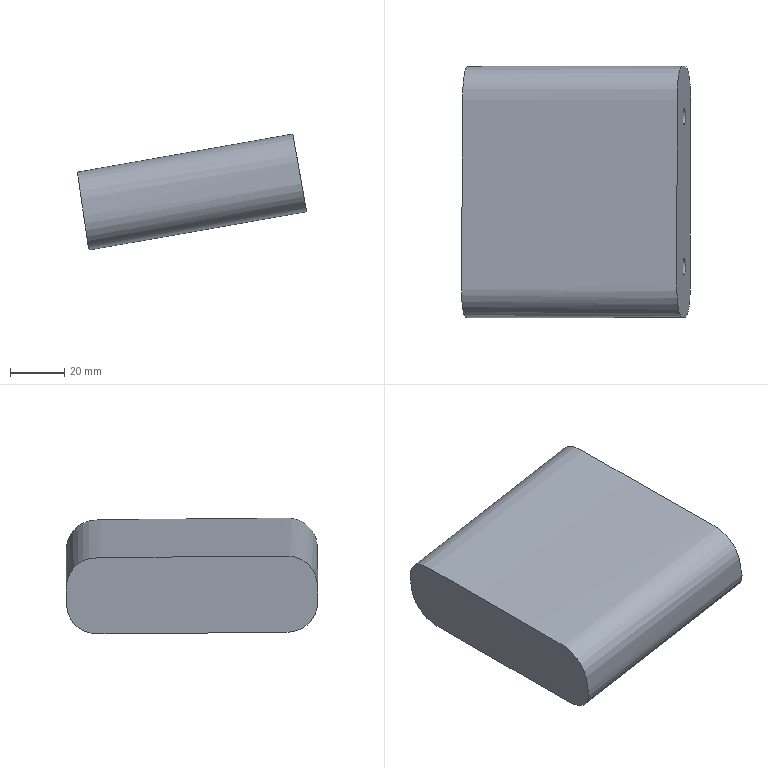Part | NX | features solid 2 | 1 solid | 7 faces | box 84.154 x 92.388 x 42.586 mm | volume 188739 mm3 | spline 2 | cone 2 | cylinder 2 | plane 1 | commonest cylinder face diameters 6 x2